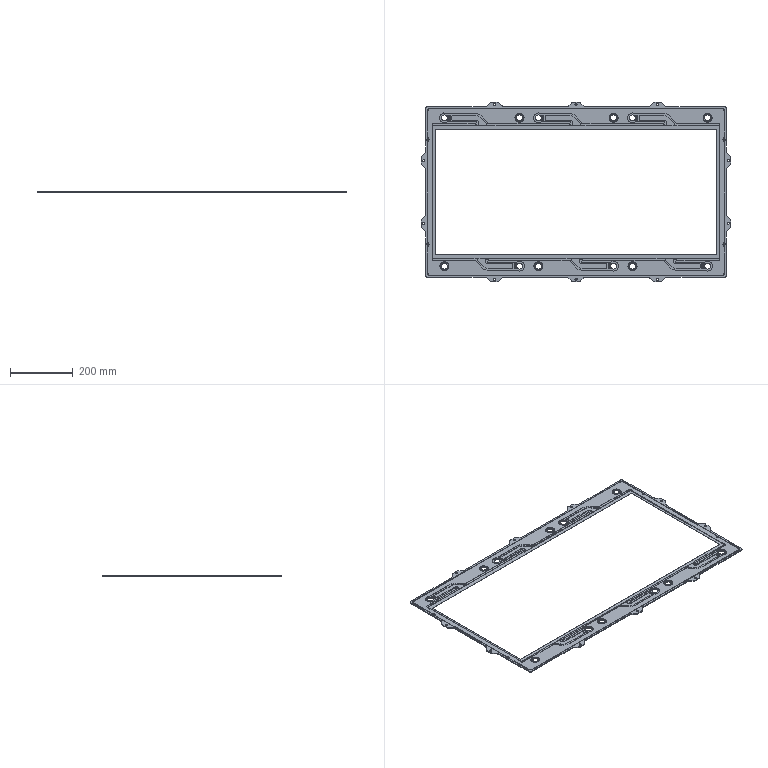Part | STEP file | Membrane frame | 1 solid | 630 faces | box 988 x 574 x 3 mm | volume 383465 mm3 | cylinder 326 | plane 304 | commonest cylinder face diameters 20 x54 7 x36 26 x33 29 x33 1 x27 19 x24